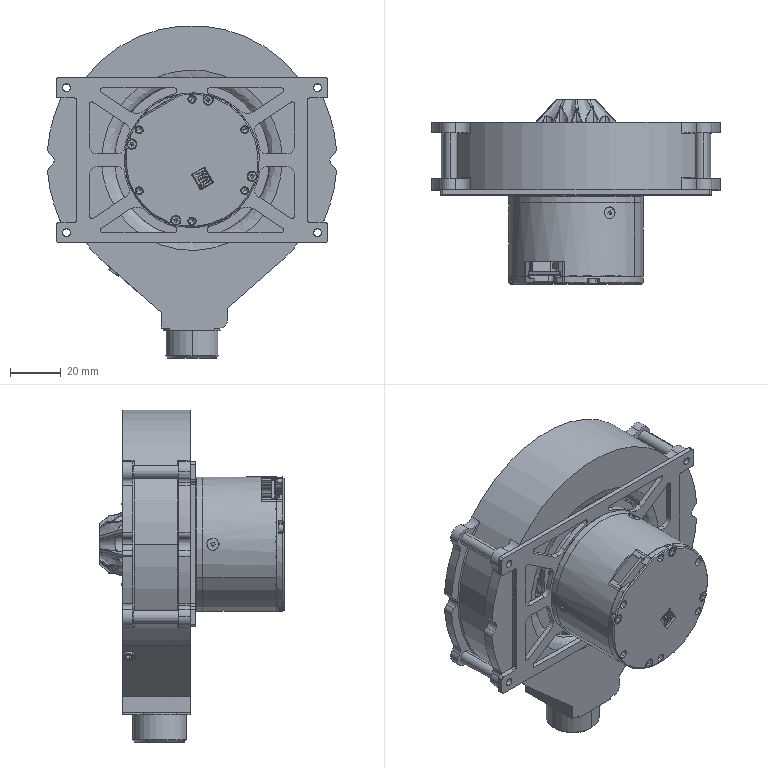Part | SolidWorks | 30 solids | 1851 faces | box 113.626 x 72.5 x 130.8 mm | volume 166546 mm3 | cylinder 1064 | plane 445 | spline 159 | cone 154 | torus 25 | sphere 4 | commonest cylinder face diameters 4 x181 5 x98 3.1 x84 2 x81 3.8 x44 2.5 x42